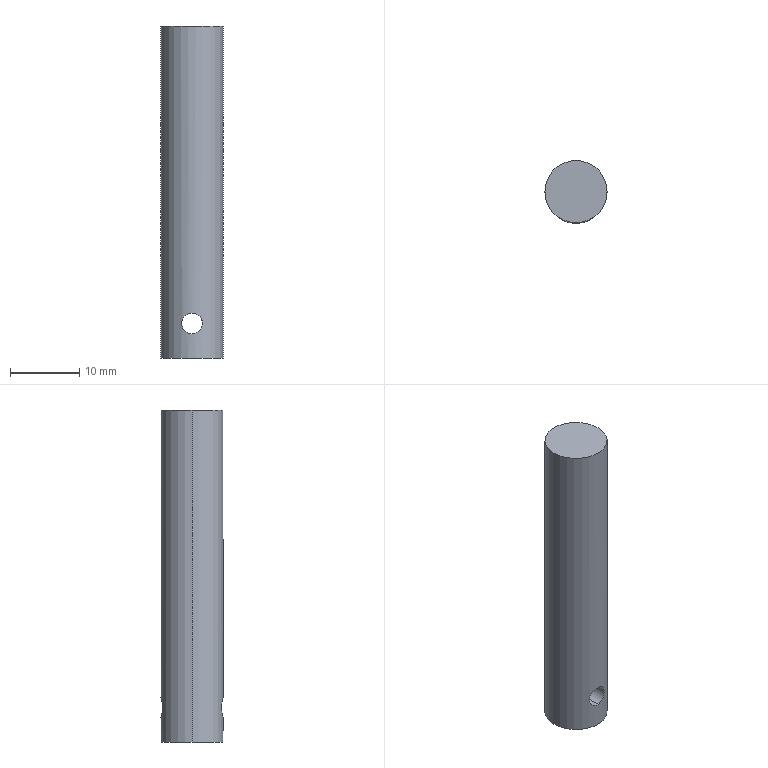Part | STEP file | Locking lead screw SGN-2-30 | 1 solid | 6 faces | box 9 x 9 x 48 mm | volume 2991 mm3 | cylinder 4 | plane 2 | commonest cylinder face diameters 3 x2 9 x2
STEP:
#1=CARTESIAN_POINT('',(0.,0.,0.));
#2=DIRECTION('',(0.,0.,1.));
#3=DIRECTION('',(1.,0.,0.));
#4=AXIS2_PLACEMENT_3D('',#1,#2,#3);
#5=CARTESIAN_POINT('',(0.,-4.5,6.5));
#6=VERTEX_POINT('',#5);
#7=CARTESIAN_POINT('',(0.,4.5,6.5));
#8=VERTEX_POINT('',#7);
#9=CARTESIAN_POINT('',(0.,-15.,6.5));
#10=DIRECTION('',(0.,1.,0.));
#11=VECTOR('',#10,1.);
#12=LINE('',#9,#11);
#13=CARTESIAN_POINT('',(0.,-15.,5.));
#14=DIRECTION('',(0.,1.,0.));
#15=DIRECTION('',(0.,0.,1.));
#16=AXIS2_PLACEMENT_3D('',#13,#14,#15);
#17=CYLINDRICAL_SURFACE('',#16,1.5);
#18=CARTESIAN_POINT('',(6.283,0.));
#19=DIRECTION('',(0.,1.));
#20=VECTOR('',#19,1.);
#21=LINE('',#18,#20);
#22=(GEOMETRIC_REPRESENTATION_CONTEXT(2)PARAMETRIC_REPRESENTATION_CONTEXT()REPRESENTATION_CONTEXT('',''));
#23=DEFINITIONAL_REPRESENTATION('',(#21),#22);
#24=PCURVE('',#17,#23);
#25=CARTESIAN_POINT('',(0.,-15.,5.));
#26=DIRECTION('',(0.,1.,0.));
#27=DIRECTION('',(0.,0.,1.));
#28=AXIS2_PLACEMENT_3D('',#25,#26,#27);
#29=CYLINDRICAL_SURFACE('',#28,1.5);
#30=CARTESIAN_POINT('',(0.,0.));
#31=DIRECTION('',(0.,1.));
#32=VECTOR('',#31,1.);
#33=LINE('',#30,#32);
#34=(GEOMETRIC_REPRESENTATION_CONTEXT(2)PARAMETRIC_REPRESENTATION_CONTEXT()REPRESENTATION_CONTEXT('',''));
#35=DEFINITIONAL_REPRESENTATION('',(#33),#34);
#36=PCURVE('',#29,#35);
#37=SURFACE_CURVE('',#12,(#24,#36),.PCURVE_S1.);
#38=EDGE_CURVE('',#6,#8,#37,.T.);
#39=ORIENTED_EDGE('',*,*,#38,.T.);
#40=CARTESIAN_POINT('',(0.,4.5,3.5));
#41=VERTEX_POINT('',#40);
#42=CARTESIAN_POINT('',(0.,4.5,6.5));
#43=CARTESIAN_POINT('',(-0.09988,4.5,6.5));
#44=CARTESIAN_POINT('',(-0.198,4.497,6.49));
#45=CARTESIAN_POINT('',(-0.3907,4.484,6.452));
#46=CARTESIAN_POINT('',(-0.4864,4.475,6.422));
#47=CARTESIAN_POINT('',(-0.7584,4.439,6.309));
#48=CARTESIAN_POINT('',(-0.9239,4.406,6.198));
#49=CARTESIAN_POINT('',(-1.198,4.34,5.923));
#50=CARTESIAN_POINT('',(-1.31,4.306,5.757));
#51=CARTESIAN_POINT('',(-1.46,4.257,5.396));
#52=CARTESIAN_POINT('',(-1.5,4.243,5.198));
#53=CARTESIAN_POINT('',(-1.5,4.243,4.902));
#54=CARTESIAN_POINT('',(-1.49,4.246,4.802));
#55=CARTESIAN_POINT('',(-1.451,4.26,4.609));
#56=CARTESIAN_POINT('',(-1.423,4.269,4.515));
#57=CARTESIAN_POINT('',(-1.309,4.306,4.241));
#58=CARTESIAN_POINT('',(-1.198,4.34,4.077));
#59=CARTESIAN_POINT('',(-0.9912,4.39,3.87));
#60=CARTESIAN_POINT('',(-0.9162,4.407,3.808));
#61=CARTESIAN_POINT('',(-0.7541,4.437,3.7));
#62=CARTESIAN_POINT('',(-0.6663,4.451,3.653));
#63=CARTESIAN_POINT('',(-0.3954,4.486,3.54));
#64=CARTESIAN_POINT('',(-0.1968,4.5,3.5));
#65=CARTESIAN_POINT('',(0.,4.5,3.5));
#66=B_SPLINE_CURVE_WITH_KNOTS('',3,(#42,#43,#44,#45,#46,#47,#48,#49,#50,#51,#52,#53,#54,#55,#56,#57,#58,#59,#60,#61,#62,#63,#64,#65),.UNSPECIFIED.,.F.,.F.,(4,2,2,2,2,2,2,2,2,2,2,4),(0.,0.0002952,0.0005905,0.001181,0.001771,0.002362,0.002657,0.002952,0.003543,0.003838,0.004133,0.004724),.UNSPECIFIED.);
#67=CARTESIAN_POINT('',(6.283,19.5));
#68=CARTESIAN_POINT('',(6.259,19.5));
#69=CARTESIAN_POINT('',(6.211,19.499));
#70=CARTESIAN_POINT('',(6.139,19.495));
#71=CARTESIAN_POINT('',(6.068,19.489));
#72=CARTESIAN_POINT('',(5.996,19.48));
#73=CARTESIAN_POINT('',(5.924,19.469));
#74=CARTESIAN_POINT('',(5.853,19.457));
#75=CARTESIAN_POINT('',(5.781,19.442));
#76=CARTESIAN_POINT('',(5.71,19.426));
#77=CARTESIAN_POINT('',(5.639,19.409));
#78=CARTESIAN_POINT('',(5.568,19.391));
#79=CARTESIAN_POINT('',(5.497,19.373));
#80=CARTESIAN_POINT('',(5.427,19.355));
#81=CARTESIAN_POINT('',(5.356,19.337));
#82=CARTESIAN_POINT('',(5.285,19.32));
#83=CARTESIAN_POINT('',(5.213,19.303));
#84=CARTESIAN_POINT('',(5.142,19.288));
#85=CARTESIAN_POINT('',(5.071,19.275));
#86=CARTESIAN_POINT('',(5.,19.264));
#87=CARTESIAN_POINT('',(4.928,19.255));
#88=CARTESIAN_POINT('',(4.857,19.248));
#89=CARTESIAN_POINT('',(4.785,19.244));
#90=CARTESIAN_POINT('',(4.713,19.242));
#91=CARTESIAN_POINT('',(4.641,19.244));
#92=CARTESIAN_POINT('',(4.568,19.248));
#93=CARTESIAN_POINT('',(4.497,19.254));
#94=CARTESIAN_POINT('',(4.425,19.263));
#95=CARTESIAN_POINT('',(4.354,19.275));
#96=CARTESIAN_POINT('',(4.282,19.288));
#97=CARTESIAN_POINT('',(4.211,19.303));
#98=CARTESIAN_POINT('',(4.139,19.32));
#99=CARTESIAN_POINT('',(4.068,19.337));
#100=CARTESIAN_POINT('',(3.998,19.355));
#101=CARTESIAN_POINT('',(3.927,19.373));
#102=CARTESIAN_POINT('',(3.856,19.392));
#103=CARTESIAN_POINT('',(3.785,19.409));
#104=CARTESIAN_POINT('',(3.714,19.426));
#105=CARTESIAN_POINT('',(3.643,19.442));
#106=CARTESIAN_POINT('',(3.571,19.457));
#107=CARTESIAN_POINT('',(3.5,19.469));
#108=CARTESIAN_POINT('',(3.429,19.48));
#109=CARTESIAN_POINT('',(3.357,19.489));
#110=CARTESIAN_POINT('',(3.285,19.495));
#111=CARTESIAN_POINT('',(3.213,19.499));
#112=CARTESIAN_POINT('',(3.165,19.5));
#113=CARTESIAN_POINT('',(3.142,19.5));
#114=B_SPLINE_CURVE_WITH_KNOTS('',3,(#67,#68,#69,#70,#71,#72,#73,#74,#75,#76,#77,#78,#79,#80,#81,#82,#83,#84,#85,#86,#87,#88,#89,#90,#91,#92,#93,#94,#95,#96,#97,#98,#99,#100,#101,#102,#103,#104,#105,#106,#107,#108,#109,#110,#111,#112,#113),.UNSPECIFIED.,.F.,.F.,(4,1,1,1,1,1,1,1,1,1,1,1,1,1,1,1,1,1,1,1,1,1,1,1,1,1,1,1,1,1,1,1,1,1,1,1,1,1,1,1,1,1,1,1,4),(0.,0.0001074,0.0002147,0.0003221,0.0004294,0.0005368,0.0006441,0.0007515,0.0008589,0.0009662,0.001074,0.001181,0.001288,0.001396,0.001503,0.00161,0.001718,0.001825,0.001932,0.00204,0.002147,0.002255,0.002362,0.002469,0.002577,0.002684,0.002791,0.002899,0.003006,0.003113,0.003221,0.003328,0.003435,0.003543,0.00365,0.003758,0.003865,0.003972,0.00408,0.004187,0.004294,0.004402,0.004509,0.004616,0.004724),.QUASI_UNIFORM_KNOTS.);
#115=(GEOMETRIC_REPRESENTATION_CONTEXT(2)PARAMETRIC_REPRESENTATION_CONTEXT()REPRESENTATION_CONTEXT('',''));
#116=DEFINITIONAL_REPRESENTATION('',(#114),#115);
#117=PCURVE('',#17,#116);
#118=CARTESIAN_POINT('',(0.,0.,48.));
#119=DIRECTION('',(0.,0.,-1.));
#120=DIRECTION('',(-1.,0.,0.));
#121=AXIS2_PLACEMENT_3D('',#118,#119,#120);
#122=CYLINDRICAL_SURFACE('',#121,4.5);
#123=CARTESIAN_POINT('',(1.571,41.5));
#124=CARTESIAN_POINT('',(1.563,41.5));
#125=CARTESIAN_POINT('',(1.547,41.503));
#126=CARTESIAN_POINT('',(1.523,41.514));
#127=CARTESIAN_POINT('',(1.499,41.533));
#128=CARTESIAN_POINT('',(1.476,41.56));
#129=CARTESIAN_POINT('',(1.453,41.595));
#130=CARTESIAN_POINT('',(1.431,41.636));
#131=CARTESIAN_POINT('',(1.41,41.684));
#132=CARTESIAN_POINT('',(1.389,41.739));
#133=CARTESIAN_POINT('',(1.369,41.8));
#134=CARTESIAN_POINT('',(1.35,41.867));
#135=CARTESIAN_POINT('',(1.333,41.939));
#136=CARTESIAN_POINT('',(1.316,42.017));
#137=CARTESIAN_POINT('',(1.301,42.1));
#138=CARTESIAN_POINT('',(1.287,42.187));
#139=CARTESIAN_POINT('',(1.274,42.279));
#140=CARTESIAN_POINT('',(1.263,42.374));
#141=CARTESIAN_POINT('',(1.253,42.472));
#142=CARTESIAN_POINT('',(1.245,42.574));
#143=CARTESIAN_POINT('',(1.239,42.678));
#144=CARTESIAN_POINT('',(1.234,42.784));
#145=CARTESIAN_POINT('',(1.232,42.892));
#146=CARTESIAN_POINT('',(1.231,42.999));
#147=CARTESIAN_POINT('',(1.232,43.107));
#148=CARTESIAN_POINT('',(1.234,43.215));
#149=CARTESIAN_POINT('',(1.239,43.321));
#150=CARTESIAN_POINT('',(1.245,43.425));
#151=CARTESIAN_POINT('',(1.253,43.527));
#152=CARTESIAN_POINT('',(1.263,43.626));
#153=CARTESIAN_POINT('',(1.274,43.722));
#154=CARTESIAN_POINT('',(1.287,43.814));
#155=CARTESIAN_POINT('',(1.301,43.901));
#156=CARTESIAN_POINT('',(1.316,43.984));
#157=CARTESIAN_POINT('',(1.333,44.062));
#158=CARTESIAN_POINT('',(1.351,44.134));
#159=CARTESIAN_POINT('',(1.369,44.201));
#160=CARTESIAN_POINT('',(1.389,44.262));
#161=CARTESIAN_POINT('',(1.41,44.316));
#162=CARTESIAN_POINT('',(1.431,44.365));
#163=CARTESIAN_POINT('',(1.453,44.406));
#164=CARTESIAN_POINT('',(1.476,44.44));
#165=CARTESIAN_POINT('',(1.499,44.466));
#166=CARTESIAN_POINT('',(1.523,44.486));
#167=CARTESIAN_POINT('',(1.547,44.497));
#168=CARTESIAN_POINT('',(1.563,44.5));
#169=CARTESIAN_POINT('',(1.571,44.5));
#170=B_SPLINE_CURVE_WITH_KNOTS('',3,(#123,#124,#125,#126,#127,#128,#129,#130,#131,#132,#133,#134,#135,#136,#137,#138,#139,#140,#141,#142,#143,#144,#145,#146,#147,#148,#149,#150,#151,#152,#153,#154,#155,#156,#157,#158,#159,#160,#161,#162,#163,#164,#165,#166,#167,#168,#169),.UNSPECIFIED.,.F.,.F.,(4,1,1,1,1,1,1,1,1,1,1,1,1,1,1,1,1,1,1,1,1,1,1,1,1,1,1,1,1,1,1,1,1,1,1,1,1,1,1,1,1,1,1,1,4),(0.,0.0001074,0.0002147,0.0003221,0.0004294,0.0005368,0.0006441,0.0007515,0.0008589,0.0009662,0.001074,0.001181,0.001288,0.001396,0.001503,0.00161,0.001718,0.001825,0.001932,0.00204,0.002147,0.002255,0.002362,0.002469,0.002577,0.002684,0.002791,0.002899,0.003006,0.003113,0.003221,0.003328,0.003435,0.003543,0.00365,0.003758,0.003865,0.003972,0.00408,0.004187,0.004294,0.004402,0.004509,0.004616,0.004724),.QUASI_UNIFORM_KNOTS.);
#171=(GEOMETRIC_REPRESENTATION_CONTEXT(2)PARAMETRIC_REPRESENTATION_CONTEXT()REPRESENTATION_CONTEXT('',''));
#172=DEFINITIONAL_REPRESENTATION('',(#170),#171);
#173=PCURVE('',#122,#172);
#174=SURFACE_CURVE('',#66,(#117,#173),.PCURVE_S1.);
#175=EDGE_CURVE('',#8,#41,#174,.T.);
#176=ORIENTED_EDGE('',*,*,#175,.T.);
#177=CARTESIAN_POINT('',(0.,-4.5,3.5));
#178=VERTEX_POINT('',#177);
#179=CARTESIAN_POINT('',(0.,-15.,3.5));
#180=DIRECTION('',(0.,1.,0.));
#181=VECTOR('',#180,1.);
#182=LINE('',#179,#181);
#183=CARTESIAN_POINT('',(3.142,0.));
#184=DIRECTION('',(0.,1.));
#185=VECTOR('',#184,1.);
#186=LINE('',#183,#185);
#187=(GEOMETRIC_REPRESENTATION_CONTEXT(2)PARAMETRIC_REPRESENTATION_CONTEXT()REPRESENTATION_CONTEXT('',''));
#188=DEFINITIONAL_REPRESENTATION('',(#186),#187);
#189=PCURVE('',#17,#188);
#190=CARTESIAN_POINT('',(3.142,0.));
#191=DIRECTION('',(0.,1.));
#192=VECTOR('',#191,1.);
#193=LINE('',#190,#192);
#194=(GEOMETRIC_REPRESENTATION_CONTEXT(2)PARAMETRIC_REPRESENTATION_CONTEXT()REPRESENTATION_CONTEXT('',''));
#195=DEFINITIONAL_REPRESENTATION('',(#193),#194);
#196=PCURVE('',#29,#195);
#197=SURFACE_CURVE('',#182,(#189,#196),.PCURVE_S1.);
#198=EDGE_CURVE('',#178,#41,#197,.T.);
#199=ORIENTED_EDGE('',*,*,#198,.F.);
#200=CARTESIAN_POINT('',(0.,-4.5,3.5));
#201=CARTESIAN_POINT('',(-0.1967,-4.5,3.5));
#202=CARTESIAN_POINT('',(-0.3953,-4.486,3.54));
#203=CARTESIAN_POINT('',(-0.6668,-4.451,3.653));
#204=CARTESIAN_POINT('',(-0.7546,-4.437,3.7));
#205=CARTESIAN_POINT('',(-0.9165,-4.406,3.809));
#206=CARTESIAN_POINT('',(-0.9916,-4.39,3.87));
#207=CARTESIAN_POINT('',(-1.199,-4.34,4.078));
#208=CARTESIAN_POINT('',(-1.309,-4.306,4.242));
#209=CARTESIAN_POINT('',(-1.423,-4.269,4.515));
#210=CARTESIAN_POINT('',(-1.451,-4.26,4.609));
#211=CARTESIAN_POINT('',(-1.49,-4.246,4.801));
#212=CARTESIAN_POINT('',(-1.5,-4.243,4.901));
#213=CARTESIAN_POINT('',(-1.5,-4.243,5.099));
#214=CARTESIAN_POINT('',(-1.49,-4.246,5.197));
#215=CARTESIAN_POINT('',(-1.452,-4.259,5.391));
#216=CARTESIAN_POINT('',(-1.422,-4.269,5.486));
#217=CARTESIAN_POINT('',(-1.31,-4.306,5.757));
#218=CARTESIAN_POINT('',(-1.198,-4.34,5.923));
#219=CARTESIAN_POINT('',(-0.9921,-4.39,6.129));
#220=CARTESIAN_POINT('',(-0.9155,-4.407,6.192));
#221=CARTESIAN_POINT('',(-0.7534,-4.437,6.301));
#222=CARTESIAN_POINT('',(-0.6676,-4.451,6.347));
#223=CARTESIAN_POINT('',(-0.4863,-4.475,6.422));
#224=CARTESIAN_POINT('',(-0.3906,-4.484,6.452));
#225=CARTESIAN_POINT('',(-0.198,-4.497,6.49));
#226=CARTESIAN_POINT('',(-0.09985,-4.5,6.5));
#227=CARTESIAN_POINT('',(0.,-4.5,6.5));
#228=B_SPLINE_CURVE_WITH_KNOTS('',3,(#200,#201,#202,#203,#204,#205,#206,#207,#208,#209,#210,#211,#212,#213,#214,#215,#216,#217,#218,#219,#220,#221,#222,#223,#224,#225,#226,#227),.UNSPECIFIED.,.F.,.F.,(4,2,2,2,2,2,2,2,2,2,2,2,2,4),(0.004724,0.005314,0.005609,0.005904,0.006495,0.00679,0.007085,0.00738,0.007675,0.008266,0.008561,0.008856,0.009151,0.009446),.UNSPECIFIED.);
#229=CARTESIAN_POINT('',(3.142,10.5));
#230=CARTESIAN_POINT('',(3.157,10.5));
#231=CARTESIAN_POINT('',(3.189,10.5));
#232=CARTESIAN_POINT('',(3.237,10.502));
#233=CARTESIAN_POINT('',(3.285,10.505));
#234=CARTESIAN_POINT('',(3.333,10.509));
#235=CARTESIAN_POINT('',(3.381,10.514));
#236=CARTESIAN_POINT('',(3.429,10.52));
#237=CARTESIAN_POINT('',(3.476,10.527));
#238=CARTESIAN_POINT('',(3.524,10.535));
#239=CARTESIAN_POINT('',(3.572,10.544));
#240=CARTESIAN_POINT('',(3.619,10.553));
#241=CARTESIAN_POINT('',(3.667,10.563));
#242=CARTESIAN_POINT('',(3.715,10.574));
#243=CARTESIAN_POINT('',(3.762,10.585));
#244=CARTESIAN_POINT('',(3.809,10.597));
#245=CARTESIAN_POINT('',(3.856,10.609));
#246=CARTESIAN_POINT('',(3.903,10.621));
#247=CARTESIAN_POINT('',(3.951,10.633));
#248=CARTESIAN_POINT('',(3.998,10.645));
#249=CARTESIAN_POINT('',(4.046,10.657));
#250=CARTESIAN_POINT('',(4.093,10.669));
#251=CARTESIAN_POINT('',(4.14,10.68));
#252=CARTESIAN_POINT('',(4.187,10.691));
#253=CARTESIAN_POINT('',(4.235,10.702));
#254=CARTESIAN_POINT('',(4.282,10.712));
#255=CARTESIAN_POINT('',(4.33,10.721));
#256=CARTESIAN_POINT('',(4.378,10.729));
#257=CARTESIAN_POINT('',(4.425,10.736));
#258=CARTESIAN_POINT('',(4.473,10.743));
#259=CARTESIAN_POINT('',(4.52,10.748));
#260=CARTESIAN_POINT('',(4.568,10.752));
#261=CARTESIAN_POINT('',(4.616,10.755));
#262=CARTESIAN_POINT('',(4.664,10.757));
#263=CARTESIAN_POINT('',(4.713,10.758));
#264=CARTESIAN_POINT('',(4.76,10.757));
#265=CARTESIAN_POINT('',(4.808,10.755));
#266=CARTESIAN_POINT('',(4.856,10.752));
#267=CARTESIAN_POINT('',(4.904,10.748));
#268=CARTESIAN_POINT('',(4.951,10.743));
#269=CARTESIAN_POINT('',(4.999,10.736));
#270=CARTESIAN_POINT('',(5.047,10.729));
#271=CARTESIAN_POINT('',(5.095,10.721));
#272=CARTESIAN_POINT('',(5.142,10.712));
#273=CARTESIAN_POINT('',(5.19,10.702));
#274=CARTESIAN_POINT('',(5.237,10.691));
#275=CARTESIAN_POINT('',(5.285,10.68));
#276=CARTESIAN_POINT('',(5.332,10.669));
#277=CARTESIAN_POINT('',(5.38,10.657));
#278=CARTESIAN_POINT('',(5.427,10.645));
#279=CARTESIAN_POINT('',(5.474,10.633));
#280=CARTESIAN_POINT('',(5.521,10.621));
#281=CARTESIAN_POINT('',(5.569,10.609));
#282=CARTESIAN_POINT('',(5.616,10.597));
#283=CARTESIAN_POINT('',(5.664,10.585));
#284=CARTESIAN_POINT('',(5.711,10.574));
#285=CARTESIAN_POINT('',(5.758,10.563));
#286=CARTESIAN_POINT('',(5.805,10.553));
#287=CARTESIAN_POINT('',(5.853,10.544));
#288=CARTESIAN_POINT('',(5.9,10.535));
#289=CARTESIAN_POINT('',(5.948,10.527));
#290=CARTESIAN_POINT('',(5.996,10.52));
#291=CARTESIAN_POINT('',(6.044,10.514));
#292=CARTESIAN_POINT('',(6.092,10.509));
#293=CARTESIAN_POINT('',(6.139,10.505));
#294=CARTESIAN_POINT('',(6.187,10.502));
#295=CARTESIAN_POINT('',(6.235,10.5));
#296=CARTESIAN_POINT('',(6.267,10.5));
#297=CARTESIAN_POINT('',(6.283,10.5));
#298=B_SPLINE_CURVE_WITH_KNOTS('',3,(#229,#230,#231,#232,#233,#234,#235,#236,#237,#238,#239,#240,#241,#242,#243,#244,#245,#246,#247,#248,#249,#250,#251,#252,#253,#254,#255,#256,#257,#258,#259,#260,#261,#262,#263,#264,#265,#266,#267,#268,#269,#270,#271,#272,#273,#274,#275,#276,#277,#278,#279,#280,#281,#282,#283,#284,#285,#286,#287,#288,#289,#290,#291,#292,#293,#294,#295,#296,#297),.UNSPECIFIED.,.F.,.F.,(4,1,1,1,1,1,1,1,1,1,1,1,1,1,1,1,1,1,1,1,1,1,1,1,1,1,1,1,1,1,1,1,1,1,1,1,1,1,1,1,1,1,1,1,1,1,1,1,1,1,1,1,1,1,1,1,1,1,1,1,1,1,1,1,1,1,4),(0.004724,0.004795,0.004867,0.004938,0.00501,0.005082,0.005153,0.005225,0.005296,0.005368,0.005439,0.005511,0.005582,0.005654,0.005725,0.005797,0.005869,0.00594,0.006012,0.006083,0.006155,0.006226,0.006298,0.006369,0.006441,0.006513,0.006584,0.006656,0.006727,0.006799,0.00687,0.006942,0.007013,0.007085,0.007157,0.007228,0.0073,0.007371,0.007443,0.007514,0.007586,0.007657,0.007729,0.007801,0.007872,0.007944,0.008015,0.008087,0.008158,0.00823,0.008301,0.008373,0.008445,0.008516,0.008588,0.008659,0.008731,0.008802,0.008874,0.008945,0.009017,0.009089,0.00916,0.009232,0.009303,0.009375,0.009446),.QUASI_UNIFORM_KNOTS.);
#299=(GEOMETRIC_REPRESENTATION_CONTEXT(2)PARAMETRIC_REPRESENTATION_CONTEXT()REPRESENTATION_CONTEXT('',''));
#300=DEFINITIONAL_REPRESENTATION('',(#298),#299);
#301=PCURVE('',#17,#300);
#302=CARTESIAN_POINT('',(0.,0.,48.));
#303=DIRECTION('',(0.,0.,-1.));
#304=DIRECTION('',(-1.,0.,0.));
#305=AXIS2_PLACEMENT_3D('',#302,#303,#304);
#306=CYLINDRICAL_SURFACE('',#305,4.5);
#307=CARTESIAN_POINT('',(4.712,44.5));
#308=CARTESIAN_POINT('',(4.718,44.5));
#309=CARTESIAN_POINT('',(4.728,44.499));
#310=CARTESIAN_POINT('',(4.744,44.494));
#311=CARTESIAN_POINT('',(4.76,44.485));
#312=CARTESIAN_POINT('',(4.776,44.473));
#313=CARTESIAN_POINT('',(4.791,44.458));
#314=CARTESIAN_POINT('',(4.807,44.439));
#315=CARTESIAN_POINT('',(4.822,44.417));
#316=CARTESIAN_POINT('',(4.837,44.392));
#317=CARTESIAN_POINT('',(4.852,44.364));
#318=CARTESIAN_POINT('',(4.866,44.332));
#319=CARTESIAN_POINT('',(4.88,44.298));
#320=CARTESIAN_POINT('',(4.894,44.261));
#321=CARTESIAN_POINT('',(4.907,44.221));
#322=CARTESIAN_POINT('',(4.92,44.179));
#323=CARTESIAN_POINT('',(4.933,44.133));
#324=CARTESIAN_POINT('',(4.945,44.086));
#325=CARTESIAN_POINT('',(4.956,44.035));
#326=CARTESIAN_POINT('',(4.967,43.983));
#327=CARTESIAN_POINT('',(4.978,43.928));
#328=CARTESIAN_POINT('',(4.987,43.871));
#329=CARTESIAN_POINT('',(4.997,43.813));
#330=CARTESIAN_POINT('',(5.005,43.752));
#331=CARTESIAN_POINT('',(5.013,43.69));
#332=CARTESIAN_POINT('',(5.02,43.626));
#333=CARTESIAN_POINT('',(5.027,43.56));
#334=CARTESIAN_POINT('',(5.033,43.493));
#335=CARTESIAN_POINT('',(5.038,43.425));
#336=CARTESIAN_POINT('',(5.042,43.356));
#337=CARTESIAN_POINT('',(5.046,43.286));
#338=CARTESIAN_POINT('',(5.049,43.216));
#339=CARTESIAN_POINT('',(5.051,43.144));
#340=CARTESIAN_POINT('',(5.052,43.072));
#341=CARTESIAN_POINT('',(5.052,43.));
#342=CARTESIAN_POINT('',(5.052,42.928));
#343=CARTESIAN_POINT('',(5.051,42.857));
#344=CARTESIAN_POINT('',(5.049,42.786));
#345=CARTESIAN_POINT('',(5.046,42.715));
#346=CARTESIAN_POINT('',(5.042,42.645));
#347=CARTESIAN_POINT('',(5.038,42.575));
#348=CARTESIAN_POINT('',(5.033,42.507));
#349=CARTESIAN_POINT('',(5.027,42.44));
#350=CARTESIAN_POINT('',(5.02,42.374));
#351=CARTESIAN_POINT('',(5.013,42.31));
#352=CARTESIAN_POINT('',(5.005,42.248));
#353=CARTESIAN_POINT('',(4.996,42.187));
#354=CARTESIAN_POINT('',(4.987,42.128));
#355=CARTESIAN_POINT('',(4.977,42.072));
#356=CARTESIAN_POINT('',(4.967,42.017));
#357=CARTESIAN_POINT('',(4.956,41.964));
#358=CARTESIAN_POINT('',(4.945,41.914));
#359=CARTESIAN_POINT('',(4.933,41.867));
#360=CARTESIAN_POINT('',(4.92,41.821));
#361=CARTESIAN_POINT('',(4.907,41.778));
#362=CARTESIAN_POINT('',(4.894,41.738));
#363=CARTESIAN_POINT('',(4.88,41.702));
#364=CARTESIAN_POINT('',(4.866,41.667));
#365=CARTESIAN_POINT('',(4.852,41.636));
#366=CARTESIAN_POINT('',(4.837,41.608));
#367=CARTESIAN_POINT('',(4.822,41.583));
#368=CARTESIAN_POINT('',(4.807,41.561));
#369=CARTESIAN_POINT('',(4.791,41.542));
#370=CARTESIAN_POINT('',(4.776,41.527));
#371=CARTESIAN_POINT('',(4.76,41.515));
#372=CARTESIAN_POINT('',(4.744,41.506));
#373=CARTESIAN_POINT('',(4.728,41.501));
#374=CARTESIAN_POINT('',(4.718,41.5));
#375=CARTESIAN_POINT('',(4.712,41.5));
#376=B_SPLINE_CURVE_WITH_KNOTS('',3,(#307,#308,#309,#310,#311,#312,#313,#314,#315,#316,#317,#318,#319,#320,#321,#322,#323,#324,#325,#326,#327,#328,#329,#330,#331,#332,#333,#334,#335,#336,#337,#338,#339,#340,#341,#342,#343,#344,#345,#346,#347,#348,#349,#350,#351,#352,#353,#354,#355,#356,#357,#358,#359,#360,#361,#362,#363,#364,#365,#366,#367,#368,#369,#370,#371,#372,#373,#374,#375),.UNSPECIFIED.,.F.,.F.,(4,1,1,1,1,1,1,1,1,1,1,1,1,1,1,1,1,1,1,1,1,1,1,1,1,1,1,1,1,1,1,1,1,1,1,1,1,1,1,1,1,1,1,1,1,1,1,1,1,1,1,1,1,1,1,1,1,1,1,1,1,1,1,1,1,1,4),(0.004724,0.004795,0.004867,0.004938,0.00501,0.005082,0.005153,0.005225,0.005296,0.005368,0.005439,0.005511,0.005582,0.005654,0.005725,0.005797,0.005869,0.00594,0.006012,0.006083,0.006155,0.006226,0.006298,0.006369,0.006441,0.006513,0.006584,0.006656,0.006727,0.006799,0.00687,0.006942,0.007013,0.007085,0.007157,0.007228,0.0073,0.007371,0.007443,0.007514,0.007586,0.007657,0.007729,0.007801,0.007872,0.007944,0.008015,0.008087,0.008158,0.00823,0.008301,0.008373,0.008445,0.008516,0.008588,0.008659,0.008731,0.008802,0.008874,0.008945,0.009017,0.009089,0.00916,0.009232,0.009303,0.009375,0.009446),.QUASI_UNIFORM_KNOTS.);
#377=(GEOMETRIC_REPRESENTATION_CONTEXT(2)PARAMETRIC_REPRESENTATION_CONTEXT()REPRESENTATION_CONTEXT('',''));
#378=DEFINITIONAL_REPRESENTATION('',(#376),#377);
#379=PCURVE('',#306,#378);
#380=SURFACE_CURVE('',#228,(#301,#379),.PCURVE_S1.);
#381=EDGE_CURVE('',#178,#6,#380,.T.);
#382=ORIENTED_EDGE('',*,*,#381,.T.);
#383=EDGE_LOOP('',(#39,#176,#199,#382));
#384=FACE_BOUND('',#383,.F.);
#385=ADVANCED_FACE('',(#384),#17,.F.);
#386=ORIENTED_EDGE('',*,*,#175,.T.);
#387=CARTESIAN_POINT('',(0.,4.5,3.5));
#388=CARTESIAN_POINT('',(0.1967,4.5,3.5));
#389=CARTESIAN_POINT('',(0.3953,4.486,3.54));
#390=CARTESIAN_POINT('',(0.6668,4.451,3.653));
#391=CARTESIAN_POINT('',(0.7546,4.437,3.7));
#392=CARTESIAN_POINT('',(0.9165,4.406,3.809));
#393=CARTESIAN_POINT('',(0.9916,4.39,3.87));
#394=CARTESIAN_POINT('',(1.199,4.34,4.078));
#395=CARTESIAN_POINT('',(1.309,4.306,4.242));
#396=CARTESIAN_POINT('',(1.423,4.269,4.515));
#397=CARTESIAN_POINT('',(1.451,4.26,4.609));
#398=CARTESIAN_POINT('',(1.49,4.246,4.801));
#399=CARTESIAN_POINT('',(1.5,4.243,4.901));
#400=CARTESIAN_POINT('',(1.5,4.243,5.099));
#401=CARTESIAN_POINT('',(1.49,4.246,5.197));
#402=CARTESIAN_POINT('',(1.452,4.259,5.391));
#403=CARTESIAN_POINT('',(1.422,4.269,5.486));
#404=CARTESIAN_POINT('',(1.31,4.306,5.757));
#405=CARTESIAN_POINT('',(1.198,4.34,5.923));
#406=CARTESIAN_POINT('',(0.9921,4.39,6.129));
#407=CARTESIAN_POINT('',(0.9155,4.407,6.192));
#408=CARTESIAN_POINT('',(0.7534,4.437,6.301));
#409=CARTESIAN_POINT('',(0.6676,4.451,6.347));
#410=CARTESIAN_POINT('',(0.4863,4.475,6.422));
#411=CARTESIAN_POINT('',(0.3906,4.484,6.452));
#412=CARTESIAN_POINT('',(0.198,4.497,6.49));
#413=CARTESIAN_POINT('',(0.09985,4.5,6.5));
#414=CARTESIAN_POINT('',(0.,4.5,6.5));
#415=B_SPLINE_CURVE_WITH_KNOTS('',3,(#387,#388,#389,#390,#391,#392,#393,#394,#395,#396,#397,#398,#399,#400,#401,#402,#403,#404,#405,#406,#407,#408,#409,#410,#411,#412,#413,#414),.UNSPECIFIED.,.F.,.F.,(4,2,2,2,2,2,2,2,2,2,2,2,2,4),(0.004724,0.005314,0.005609,0.005904,0.006495,0.00679,0.007085,0.00738,0.007675,0.008266,0.008561,0.008856,0.009151,0.009446),.UNSPECIFIED.);
#416=CARTESIAN_POINT('',(1.571,44.5));
#417=CARTESIAN_POINT('',(1.576,44.5));
#418=CARTESIAN_POINT('',(1.587,44.499));
#419=CARTESIAN_POINT('',(1.603,44.494));
#420=CARTESIAN_POINT('',(1.618,44.485));
#421=CARTESIAN_POINT('',(1.634,44.473));
#422=CARTESIAN_POINT('',(1.65,44.458));
#423=CARTESIAN_POINT('',(1.665,44.439));
#424=CARTESIAN_POINT('',(1.681,44.417));
#425=CARTESIAN_POINT('',(1.696,44.392));
#426=CARTESIAN_POINT('',(1.71,44.364));
#427=CARTESIAN_POINT('',(1.725,44.332));
#428=CARTESIAN_POINT('',(1.739,44.298));
#429=CARTESIAN_POINT('',(1.753,44.261));
#430=CARTESIAN_POINT('',(1.766,44.221));
#431=CARTESIAN_POINT('',(1.779,44.179));
#432=CARTESIAN_POINT('',(1.791,44.133));
#433=CARTESIAN_POINT('',(1.803,44.086));
#434=CARTESIAN_POINT('',(1.815,44.035));
#435=CARTESIAN_POINT('',(1.826,43.983));
#436=CARTESIAN_POINT('',(1.836,43.928));
#437=CARTESIAN_POINT('',(1.846,43.871));
#438=CARTESIAN_POINT('',(1.855,43.813));
#439=CARTESIAN_POINT('',(1.864,43.752));
#440=CARTESIAN_POINT('',(1.871,43.69));
#441=CARTESIAN_POINT('',(1.879,43.626));
#442=CARTESIAN_POINT('',(1.885,43.56));
#443=CARTESIAN_POINT('',(1.891,43.493));
#444=CARTESIAN_POINT('',(1.896,43.425));
#445=CARTESIAN_POINT('',(1.901,43.356));
#446=CARTESIAN_POINT('',(1.904,43.286));
#447=CARTESIAN_POINT('',(1.907,43.216));
#448=CARTESIAN_POINT('',(1.909,43.144));
#449=CARTESIAN_POINT('',(1.91,43.072));
#450=CARTESIAN_POINT('',(1.911,43.));
#451=CARTESIAN_POINT('',(1.91,42.928));
#452=CARTESIAN_POINT('',(1.909,42.857));
#453=CARTESIAN_POINT('',(1.907,42.786));
#454=CARTESIAN_POINT('',(1.904,42.715));
#455=CARTESIAN_POINT('',(1.901,42.645));
#456=CARTESIAN_POINT('',(1.896,42.575));
#457=CARTESIAN_POINT('',(1.891,42.507));
#458=CARTESIAN_POINT('',(1.885,42.44));
#459=CARTESIAN_POINT('',(1.879,42.374));
#460=CARTESIAN_POINT('',(1.871,42.31));
#461=CARTESIAN_POINT('',(1.863,42.248));
#462=CARTESIAN_POINT('',(1.855,42.187));
#463=CARTESIAN_POINT('',(1.846,42.128));
#464=CARTESIAN_POINT('',(1.836,42.072));
#465=CARTESIAN_POINT('',(1.825,42.017));
#466=CARTESIAN_POINT('',(1.815,41.964));
#467=CARTESIAN_POINT('',(1.803,41.914));
#468=CARTESIAN_POINT('',(1.791,41.867));
#469=CARTESIAN_POINT('',(1.779,41.821));
#470=CARTESIAN_POINT('',(1.766,41.778));
#471=CARTESIAN_POINT('',(1.752,41.738));
#472=CARTESIAN_POINT('',(1.739,41.702));
#473=CARTESIAN_POINT('',(1.725,41.667));
#474=CARTESIAN_POINT('',(1.71,41.636));
#475=CARTESIAN_POINT('',(1.696,41.608));
#476=CARTESIAN_POINT('',(1.681,41.583));
#477=CARTESIAN_POINT('',(1.665,41.561));
#478=CARTESIAN_POINT('',(1.65,41.542));
#479=CARTESIAN_POINT('',(1.634,41.527));
#480=CARTESIAN_POINT('',(1.619,41.515));
#481=CARTESIAN_POINT('',(1.603,41.506));
#482=CARTESIAN_POINT('',(1.587,41.501));
#483=CARTESIAN_POINT('',(1.576,41.5));
#484=CARTESIAN_POINT('',(1.571,41.5));
#485=B_SPLINE_CURVE_WITH_KNOTS('',3,(#416,#417,#418,#419,#420,#421,#422,#423,#424,#425,#426,#427,#428,#429,#430,#431,#432,#433,#434,#435,#436,#437,#438,#439,#440,#441,#442,#443,#444,#445,#446,#447,#448,#449,#450,#451,#452,#453,#454,#455,#456,#457,#458,#459,#460,#461,#462,#463,#464,#465,#466,#467,#468,#469,#470,#471,#472,#473,#474,#475,#476,#477,#478,#479,#480,#481,#482,#483,#484),.UNSPECIFIED.,.F.,.F.,(4,1,1,1,1,1,1,1,1,1,1,1,1,1,1,1,1,1,1,1,1,1,1,1,1,1,1,1,1,1,1,1,1,1,1,1,1,1,1,1,1,1,1,1,1,1,1,1,1,1,1,1,1,1,1,1,1,1,1,1,1,1,1,1,1,1,4),(0.004724,0.004795,0.004867,0.004938,0.00501,0.005082,0.005153,0.005225,0.005296,0.005368,0.005439,0.005511,0.005582,0.005654,0.005725,0.005797,0.005869,0.00594,0.006012,0.006083,0.006155,0.006226,0.006298,0.006369,0.006441,0.006513,0.006584,0.006656,0.006727,0.006799,0.00687,0.006942,0.007013,0.007085,0.007157,0.007228,0.0073,0.007371,0.007443,0.007514,0.007586,0.007657,0.007729,0.007801,0.007872,0.007944,0.008015,0.008087,0.008158,0.00823,0.008301,0.008373,0.008445,0.008516,0.008588,0.008659,0.008731,0.008802,0.008874,0.008945,0.009017,0.009089,0.00916,0.009232,0.009303,0.009375,0.009446),.QUASI_UNIFORM_KNOTS.);
#486=(GEOMETRIC_REPRESENTATION_CONTEXT(2)PARAMETRIC_REPRESENTATION_CONTEXT()REPRESENTATION_CONTEXT('',''));
#487=DEFINITIONAL_REPRESENTATION('',(#485),#486);
#488=PCURVE('',#122,#487);
#489=CARTESIAN_POINT('',(3.142,19.5));
#490=CARTESIAN_POINT('',(3.126,19.5));
#491=CARTESIAN_POINT('',(3.094,19.5));
#492=CARTESIAN_POINT('',(3.046,19.498));
#493=CARTESIAN_POINT('',(2.998,19.495));
#494=CARTESIAN_POINT('',(2.95,19.491));
#495=CARTESIAN_POINT('',(2.902,19.486));
#496=CARTESIAN_POINT('',(2.854,19.48));
#497=CARTESIAN_POINT('',(2.807,19.473));
#498=CARTESIAN_POINT('',(2.759,19.465));
#499=CARTESIAN_POINT('',(2.712,19.456));
#500=CARTESIAN_POINT('',(2.664,19.447));
#501=CARTESIAN_POINT('',(2.616,19.437));
#502=CARTESIAN_POINT('',(2.568,19.426));
#503=CARTESIAN_POINT('',(2.521,19.415));
#504=CARTESIAN_POINT('',(2.474,19.403));
#505=CARTESIAN_POINT('',(2.427,19.391));
#506=CARTESIAN_POINT('',(2.38,19.379));
#507=CARTESIAN_POINT('',(2.332,19.367));
#508=CARTESIAN_POINT('',(2.285,19.355));
#509=CARTESIAN_POINT('',(2.238,19.343));
#510=CARTESIAN_POINT('',(2.19,19.331));
#511=CARTESIAN_POINT('',(2.143,19.32));
#512=CARTESIAN_POINT('',(2.096,19.309));
#513=CARTESIAN_POINT('',(2.048,19.298));
#514=CARTESIAN_POINT('',(2.001,19.288));
#515=CARTESIAN_POINT('',(1.953,19.279));
#516=CARTESIAN_POINT('',(1.905,19.271));
#517=CARTESIAN_POINT('',(1.858,19.264));
#518=CARTESIAN_POINT('',(1.81,19.257));
#519=CARTESIAN_POINT('',(1.763,19.252));
#520=CARTESIAN_POINT('',(1.715,19.248));
#521=CARTESIAN_POINT('',(1.667,19.245));
#522=CARTESIAN_POINT('',(1.619,19.243));
#523=CARTESIAN_POINT('',(1.571,19.242));
#524=CARTESIAN_POINT('',(1.523,19.243));
#525=CARTESIAN_POINT('',(1.475,19.245));
#526=CARTESIAN_POINT('',(1.427,19.248));
#527=CARTESIAN_POINT('',(1.38,19.252));
#528=CARTESIAN_POINT('',(1.332,19.257));
#529=CARTESIAN_POINT('',(1.284,19.264));
#530=CARTESIAN_POINT('',(1.236,19.271));
#531=CARTESIAN_POINT('',(1.188,19.279));
#532=CARTESIAN_POINT('',(1.141,19.288));
#533=CARTESIAN_POINT('',(1.093,19.298));
#534=CARTESIAN_POINT('',(1.046,19.309));
#535=CARTESIAN_POINT('',(0.9984,19.32));
#536=CARTESIAN_POINT('',(0.951,19.331));
#537=CARTESIAN_POINT('',(0.9037,19.343));
#538=CARTESIAN_POINT('',(0.8564,19.355));
#539=CARTESIAN_POINT('',(0.8091,19.367));
#540=CARTESIAN_POINT('',(0.762,19.379));
#541=CARTESIAN_POINT('',(0.7146,19.391));
#542=CARTESIAN_POINT('',(0.667,19.403));
#543=CARTESIAN_POINT('',(0.6195,19.415));
#544=CARTESIAN_POINT('',(0.5722,19.426));
#545=CARTESIAN_POINT('',(0.525,19.437));
#546=CARTESIAN_POINT('',(0.4778,19.447));
#547=CARTESIAN_POINT('',(0.4305,19.456));
#548=CARTESIAN_POINT('',(0.383,19.465));
#549=CARTESIAN_POINT('',(0.3351,19.473));
#550=CARTESIAN_POINT('',(0.2872,19.48));
#551=CARTESIAN_POINT('',(0.2392,19.486));
#552=CARTESIAN_POINT('',(0.1915,19.491));
#553=CARTESIAN_POINT('',(0.1439,19.495));
#554=CARTESIAN_POINT('',(0.09618,19.498));
#555=CARTESIAN_POINT('',(0.04828,19.5));
#556=CARTESIAN_POINT('',(0.01614,19.5));
#557=CARTESIAN_POINT('',(0.,19.5));
#558=B_SPLINE_CURVE_WITH_KNOTS('',3,(#489,#490,#491,#492,#493,#494,#495,#496,#497,#498,#499,#500,#501,#502,#503,#504,#505,#506,#507,#508,#509,#510,#511,#512,#513,#514,#515,#516,#517,#518,#519,#520,#521,#522,#523,#524,#525,#526,#527,#528,#529,#530,#531,#532,#533,#534,#535,#536,#537,#538,#539,#540,#541,#542,#543,#544,#545,#546,#547,#548,#549,#550,#551,#552,#553,#554,#555,#556,#557),.UNSPECIFIED.,.F.,.F.,(4,1,1,1,1,1,1,1,1,1,1,1,1,1,1,1,1,1,1,1,1,1,1,1,1,1,1,1,1,1,1,1,1,1,1,1,1,1,1,1,1,1,1,1,1,1,1,1,1,1,1,1,1,1,1,1,1,1,1,1,1,1,1,1,1,1,4),(0.004724,0.004795,0.004867,0.004938,0.00501,0.005082,0.005153,0.005225,0.005296,0.005368,0.005439,0.005511,0.005582,0.005654,0.005725,0.005797,0.005869,0.00594,0.006012,0.006083,0.006155,0.006226,0.006298,0.006369,0.006441,0.006513,0.006584,0.006656,0.006727,0.006799,0.00687,0.006942,0.007013,0.007085,0.007157,0.007228,0.0073,0.007371,0.007443,0.007514,0.007586,0.007657,0.007729,0.007801,0.007872,0.007944,0.008015,0.008087,0.008158,0.00823,0.008301,0.008373,0.008445,0.008516,0.008588,0.008659,0.008731,0.008802,0.008874,0.008945,0.009017,0.009089,0.00916,0.009232,0.009303,0.009375,0.009446),.QUASI_UNIFORM_KNOTS.);
#559=(GEOMETRIC_REPRESENTATION_CONTEXT(2)PARAMETRIC_REPRESENTATION_CONTEXT()REPRESENTATION_CONTEXT('',''));
#560=DEFINITIONAL_REPRESENTATION('',(#558),#559);
#561=PCURVE('',#29,#560);
#562=SURFACE_CURVE('',#415,(#488,#561),.PCURVE_S1.);
#563=EDGE_CURVE('',#41,#8,#562,.T.);
#564=ORIENTED_EDGE('',*,*,#563,.T.);
#565=EDGE_LOOP('',(#386,#564));
#566=FACE_BOUND('',#565,.T.);
#567=CARTESIAN_POINT('',(4.5,0.,48.));
#568=VERTEX_POINT('',#567);
#569=CARTESIAN_POINT('',(-4.5,0.,48.));
#570=VERTEX_POINT('',#569);
#571=CARTESIAN_POINT('',(0.,0.,48.));
#572=DIRECTION('',(0.,0.,1.));
#573=DIRECTION('',(1.,0.,0.));
#574=AXIS2_PLACEMENT_3D('',#571,#572,#573);
#575=CIRCLE('',#574,4.5);
#576=CARTESIAN_POINT('',(3.142,0.));
#577=DIRECTION('',(-1.,0.));
#578=VECTOR('',#577,1.);
#579=LINE('',#576,#578);
#580=(GEOMETRIC_REPRESENTATION_CONTEXT(2)PARAMETRIC_REPRESENTATION_CONTEXT()REPRESENTATION_CONTEXT('',''));
#581=DEFINITIONAL_REPRESENTATION('',(#579),#580);
#582=PCURVE('',#122,#581);
#583=CARTESIAN_POINT('',(0.,0.,48.));
#584=DIRECTION('',(0.,0.,1.));
#585=DIRECTION('',(1.,0.,0.));
#586=AXIS2_PLACEMENT_3D('',#583,#584,#585);
#587=PLANE('',#586);
#588=CARTESIAN_POINT('',(0.,0.));
#589=DIRECTION('',(1.,0.));
#590=AXIS2_PLACEMENT_2D('',#588,#589);
#591=CIRCLE('',#590,4.5);
#592=(GEOMETRIC_REPRESENTATION_CONTEXT(2)PARAMETRIC_REPRESENTATION_CONTEXT()REPRESENTATION_CONTEXT('',''));
#593=DEFINITIONAL_REPRESENTATION('',(#591),#592);
#594=PCURVE('',#587,#593);
#595=SURFACE_CURVE('',#575,(#582,#594),.PCURVE_S1.);
#596=EDGE_CURVE('',#568,#570,#595,.T.);
#597=ORIENTED_EDGE('',*,*,#596,.F.);
#598=CARTESIAN_POINT('',(4.5,0.,0.));
#599=VERTEX_POINT('',#598);
#600=CARTESIAN_POINT('',(4.5,0.,48.));
#601=DIRECTION('',(0.,0.,-1.));
#602=VECTOR('',#601,1.);
#603=LINE('',#600,#602);
#604=CARTESIAN_POINT('',(3.142,0.));
#605=DIRECTION('',(0.,1.));
#606=VECTOR('',#605,1.);
#607=LINE('',#604,#606);
#608=(GEOMETRIC_REPRESENTATION_CONTEXT(2)PARAMETRIC_REPRESENTATION_CONTEXT()REPRESENTATION_CONTEXT('',''));
#609=DEFINITIONAL_REPRESENTATION('',(#607),#608);
#610=PCURVE('',#122,#609);
#611=CARTESIAN_POINT('',(3.142,0.));
#612=DIRECTION('',(0.,1.));
#613=VECTOR('',#612,1.);
#614=LINE('',#611,#613);
#615=(GEOMETRIC_REPRESENTATION_CONTEXT(2)PARAMETRIC_REPRESENTATION_CONTEXT()REPRESENTATION_CONTEXT('',''));
#616=DEFINITIONAL_REPRESENTATION('',(#614),#615);
#617=PCURVE('',#306,#616);
#618=SURFACE_CURVE('',#603,(#610,#617),.PCURVE_S1.);
#619=EDGE_CURVE('',#568,#599,#618,.T.);
#620=ORIENTED_EDGE('',*,*,#619,.T.);
#621=CARTESIAN_POINT('',(-4.5,0.,0.));
#622=VERTEX_POINT('',#621);
#623=CARTESIAN_POINT('',(0.,0.,0.));
#624=DIRECTION('',(0.,0.,1.));
#625=DIRECTION('',(1.,0.,0.));
#626=AXIS2_PLACEMENT_3D('',#623,#624,#625);
#627=CIRCLE('',#626,4.5);
#628=CARTESIAN_POINT('',(3.142,48.));
#629=DIRECTION('',(-1.,0.));
#630=VECTOR('',#629,1.);
#631=LINE('',#628,#630);
#632=(GEOMETRIC_REPRESENTATION_CONTEXT(2)PARAMETRIC_REPRESENTATION_CONTEXT()REPRESENTATION_CONTEXT('',''));
#633=DEFINITIONAL_REPRESENTATION('',(#631),#632);
#634=PCURVE('',#122,#633);
#635=CARTESIAN_POINT('',(0.,0.,0.));
#636=DIRECTION('',(0.,0.,1.));
#637=DIRECTION('',(1.,0.,0.));
#638=AXIS2_PLACEMENT_3D('',#635,#636,#637);
#639=PLANE('',#638);
#640=CARTESIAN_POINT('',(0.,0.));
#641=DIRECTION('',(1.,0.));
#642=AXIS2_PLACEMENT_2D('',#640,#641);
#643=CIRCLE('',#642,4.5);
#644=(GEOMETRIC_REPRESENTATION_CONTEXT(2)PARAMETRIC_REPRESENTATION_CONTEXT()REPRESENTATION_CONTEXT('',''));
#645=DEFINITIONAL_REPRESENTATION('',(#643),#644);
#646=PCURVE('',#639,#645);
#647=SURFACE_CURVE('',#627,(#634,#646),.PCURVE_S1.);
#648=EDGE_CURVE('',#599,#622,#647,.T.);
#649=ORIENTED_EDGE('',*,*,#648,.T.);
#650=CARTESIAN_POINT('',(-4.5,0.,48.));
#651=DIRECTION('',(0.,0.,-1.));
#652=VECTOR('',#651,1.);
#653=LINE('',#650,#652);
#654=CARTESIAN_POINT('',(0.,0.));
#655=DIRECTION('',(0.,1.));
#656=VECTOR('',#655,1.);
#657=LINE('',#654,#656);
#658=(GEOMETRIC_REPRESENTATION_CONTEXT(2)PARAMETRIC_REPRESENTATION_CONTEXT()REPRESENTATION_CONTEXT('',''));
#659=DEFINITIONAL_REPRESENTATION('',(#657),#658);
#660=PCURVE('',#122,#659);
#661=CARTESIAN_POINT('',(6.283,0.));
#662=DIRECTION('',(0.,1.));
#663=VECTOR('',#662,1.);
#664=LINE('',#661,#663);
#665=(GEOMETRIC_REPRESENTATION_CONTEXT(2)PARAMETRIC_REPRESENTATION_CONTEXT()REPRESENTATION_CONTEXT('',''));
#666=DEFINITIONAL_REPRESENTATION('',(#664),#665);
#667=PCURVE('',#306,#666);
#668=SURFACE_CURVE('',#653,(#660,#667),.PCURVE_S1.);
#669=EDGE_CURVE('',#570,#622,#668,.T.);
#670=ORIENTED_EDGE('',*,*,#669,.F.);
#671=EDGE_LOOP('',(#597,#620,#649,#670));
#672=FACE_BOUND('',#671,.T.);
#673=ADVANCED_FACE('',(#566,#672),#122,.T.);
#674=ORIENTED_EDGE('',*,*,#619,.F.);
#675=CARTESIAN_POINT('',(0.,0.,48.));
#676=DIRECTION('',(0.,0.,1.));
#677=DIRECTION('',(1.,0.,0.));
#678=AXIS2_PLACEMENT_3D('',#675,#676,#677);
#679=CIRCLE('',#678,4.5);
#680=CARTESIAN_POINT('',(9.425,0.));
#681=DIRECTION('',(-1.,0.));
#682=VECTOR('',#681,1.);
#683=LINE('',#680,#682);
#684=(GEOMETRIC_REPRESENTATION_CONTEXT(2)PARAMETRIC_REPRESENTATION_CONTEXT()REPRESENTATION_CONTEXT('',''));
#685=DEFINITIONAL_REPRESENTATION('',(#683),#684);
#686=PCURVE('',#306,#685);
#687=CARTESIAN_POINT('',(0.,0.));
#688=DIRECTION('',(1.,0.));
#689=AXIS2_PLACEMENT_2D('',#687,#688);
#690=CIRCLE('',#689,4.5);
#691=(GEOMETRIC_REPRESENTATION_CONTEXT(2)PARAMETRIC_REPRESENTATION_CONTEXT()REPRESENTATION_CONTEXT('',''));
#692=DEFINITIONAL_REPRESENTATION('',(#690),#691);
#693=PCURVE('',#587,#692);
#694=SURFACE_CURVE('',#679,(#686,#693),.PCURVE_S1.);
#695=EDGE_CURVE('',#570,#568,#694,.T.);
#696=ORIENTED_EDGE('',*,*,#695,.F.);
#697=ORIENTED_EDGE('',*,*,#669,.T.);
#698=CARTESIAN_POINT('',(0.,0.,0.));
#699=DIRECTION('',(0.,0.,1.));
#700=DIRECTION('',(1.,0.,0.));
#701=AXIS2_PLACEMENT_3D('',#698,#699,#700);
#702=CIRCLE('',#701,4.5);
#703=CARTESIAN_POINT('',(9.425,48.));
#704=DIRECTION('',(-1.,0.));
#705=VECTOR('',#704,1.);
#706=LINE('',#703,#705);
#707=(GEOMETRIC_REPRESENTATION_CONTEXT(2)PARAMETRIC_REPRESENTATION_CONTEXT()REPRESENTATION_CONTEXT('',''));
#708=DEFINITIONAL_REPRESENTATION('',(#706),#707);
#709=PCURVE('',#306,#708);
#710=CARTESIAN_POINT('',(0.,0.));
#711=DIRECTION('',(1.,0.));
#712=AXIS2_PLACEMENT_2D('',#710,#711);
#713=CIRCLE('',#712,4.5);
#714=(GEOMETRIC_REPRESENTATION_CONTEXT(2)PARAMETRIC_REPRESENTATION_CONTEXT()REPRESENTATION_CONTEXT('',''));
#715=DEFINITIONAL_REPRESENTATION('',(#713),#714);
#716=PCURVE('',#639,#715);
#717=SURFACE_CURVE('',#702,(#709,#716),.PCURVE_S1.);
#718=EDGE_CURVE('',#622,#599,#717,.T.);
#719=ORIENTED_EDGE('',*,*,#718,.T.);
#720=EDGE_LOOP('',(#674,#696,#697,#719));
#721=FACE_BOUND('',#720,.T.);
#722=CARTESIAN_POINT('',(0.,-4.5,6.5));
#723=CARTESIAN_POINT('',(0.09988,-4.5,6.5));
#724=CARTESIAN_POINT('',(0.198,-4.497,6.49));
#725=CARTESIAN_POINT('',(0.3907,-4.484,6.452));
#726=CARTESIAN_POINT('',(0.4864,-4.475,6.422));
#727=CARTESIAN_POINT('',(0.7584,-4.439,6.309));
#728=CARTESIAN_POINT('',(0.9239,-4.406,6.198));
#729=CARTESIAN_POINT('',(1.198,-4.34,5.923));
#730=CARTESIAN_POINT('',(1.31,-4.306,5.757));
#731=CARTESIAN_POINT('',(1.46,-4.257,5.396));
#732=CARTESIAN_POINT('',(1.5,-4.243,5.198));
#733=CARTESIAN_POINT('',(1.5,-4.243,4.902));
#734=CARTESIAN_POINT('',(1.49,-4.246,4.802));
#735=CARTESIAN_POINT('',(1.451,-4.26,4.609));
#736=CARTESIAN_POINT('',(1.423,-4.269,4.515));
#737=CARTESIAN_POINT('',(1.309,-4.306,4.241));
#738=CARTESIAN_POINT('',(1.198,-4.34,4.077));
#739=CARTESIAN_POINT('',(0.9912,-4.39,3.87));
#740=CARTESIAN_POINT('',(0.9162,-4.407,3.808));
#741=CARTESIAN_POINT('',(0.7541,-4.437,3.7));
#742=CARTESIAN_POINT('',(0.6663,-4.451,3.653));
#743=CARTESIAN_POINT('',(0.3954,-4.486,3.54));
#744=CARTESIAN_POINT('',(0.1968,-4.5,3.5));
#745=CARTESIAN_POINT('',(0.,-4.5,3.5));
#746=B_SPLINE_CURVE_WITH_KNOTS('',3,(#722,#723,#724,#725,#726,#727,#728,#729,#730,#731,#732,#733,#734,#735,#736,#737,#738,#739,#740,#741,#742,#743,#744,#745),.UNSPECIFIED.,.F.,.F.,(4,2,2,2,2,2,2,2,2,2,2,4),(0.,0.0002952,0.0005905,0.001181,0.001771,0.002362,0.002657,0.002952,0.003543,0.003838,0.004133,0.004724),.UNSPECIFIED.);
#747=CARTESIAN_POINT('',(4.712,41.5));
#748=CARTESIAN_POINT('',(4.704,41.5));
#749=CARTESIAN_POINT('',(4.688,41.503));
#750=CARTESIAN_POINT('',(4.665,41.514));
#751=CARTESIAN_POINT('',(4.641,41.533));
#752=CARTESIAN_POINT('',(4.618,41.56));
#753=CARTESIAN_POINT('',(4.595,41.595));
#754=CARTESIAN_POINT('',(4.573,41.636));
#755=CARTESIAN_POINT('',(4.551,41.684));
#756=CARTESIAN_POINT('',(4.53,41.739));
#757=CARTESIAN_POINT('',(4.511,41.8));
#758=CARTESIAN_POINT('',(4.492,41.867));
#759=CARTESIAN_POINT('',(4.474,41.939));
#760=CARTESIAN_POINT('',(4.458,42.017));
#761=CARTESIAN_POINT('',(4.442,42.1));
#762=CARTESIAN_POINT('',(4.428,42.187));
#763=CARTESIAN_POINT('',(4.415,42.279));
#764=CARTESIAN_POINT('',(4.404,42.374));
#765=CARTESIAN_POINT('',(4.395,42.472));
#766=CARTESIAN_POINT('',(4.387,42.574));
#767=CARTESIAN_POINT('',(4.381,42.678));
#768=CARTESIAN_POINT('',(4.376,42.784));
#769=CARTESIAN_POINT('',(4.373,42.892));
#770=CARTESIAN_POINT('',(4.372,42.999));
#771=CARTESIAN_POINT('',(4.373,43.107));
#772=CARTESIAN_POINT('',(4.376,43.215));
#773=CARTESIAN_POINT('',(4.38,43.321));
#774=CARTESIAN_POINT('',(4.387,43.425));
#775=CARTESIAN_POINT('',(4.395,43.527));
#776=CARTESIAN_POINT('',(4.404,43.626));
#777=CARTESIAN_POINT('',(4.416,43.722));
#778=CARTESIAN_POINT('',(4.428,43.814));
#779=CARTESIAN_POINT('',(4.442,43.901));
#780=CARTESIAN_POINT('',(4.458,43.984));
#781=CARTESIAN_POINT('',(4.474,44.062));
#782=CARTESIAN_POINT('',(4.492,44.134));
#783=CARTESIAN_POINT('',(4.511,44.201));
#784=CARTESIAN_POINT('',(4.531,44.262));
#785=CARTESIAN_POINT('',(4.551,44.316));
#786=CARTESIAN_POINT('',(4.573,44.365));
#787=CARTESIAN_POINT('',(4.595,44.406));
#788=CARTESIAN_POINT('',(4.618,44.44));
#789=CARTESIAN_POINT('',(4.641,44.466));
#790=CARTESIAN_POINT('',(4.665,44.486));
#791=CARTESIAN_POINT('',(4.689,44.497));
#792=CARTESIAN_POINT('',(4.704,44.5));
#793=CARTESIAN_POINT('',(4.712,44.5));
#794=B_SPLINE_CURVE_WITH_KNOTS('',3,(#747,#748,#749,#750,#751,#752,#753,#754,#755,#756,#757,#758,#759,#760,#761,#762,#763,#764,#765,#766,#767,#768,#769,#770,#771,#772,#773,#774,#775,#776,#777,#778,#779,#780,#781,#782,#783,#784,#785,#786,#787,#788,#789,#790,#791,#792,#793),.UNSPECIFIED.,.F.,.F.,(4,1,1,1,1,1,1,1,1,1,1,1,1,1,1,1,1,1,1,1,1,1,1,1,1,1,1,1,1,1,1,1,1,1,1,1,1,1,1,1,1,1,1,1,4),(0.,0.0001074,0.0002147,0.0003221,0.0004294,0.0005368,0.0006441,0.0007515,0.0008589,0.0009662,0.001074,0.001181,0.001288,0.001396,0.001503,0.00161,0.001718,0.001825,0.001932,0.00204,0.002147,0.002255,0.002362,0.002469,0.002577,0.002684,0.002791,0.002899,0.003006,0.003113,0.003221,0.003328,0.003435,0.003543,0.00365,0.003758,0.003865,0.003972,0.00408,0.004187,0.004294,0.004402,0.004509,0.004616,0.004724),.QUASI_UNIFORM_KNOTS.);
#795=(GEOMETRIC_REPRESENTATION_CONTEXT(2)PARAMETRIC_REPRESENTATION_CONTEXT()REPRESENTATION_CONTEXT('',''));
#796=DEFINITIONAL_REPRESENTATION('',(#794),#795);
#797=PCURVE('',#306,#796);
#798=CARTESIAN_POINT('',(0.,10.5));
#799=CARTESIAN_POINT('',(0.02421,10.5));
#800=CARTESIAN_POINT('',(0.07232,10.501));
#801=CARTESIAN_POINT('',(0.1439,10.505));
#802=CARTESIAN_POINT('',(0.2153,10.511));
#803=CARTESIAN_POINT('',(0.2872,10.52));
#804=CARTESIAN_POINT('',(0.3592,10.531));
#805=CARTESIAN_POINT('',(0.4306,10.543));
#806=CARTESIAN_POINT('',(0.5019,10.558));
#807=CARTESIAN_POINT('',(0.5732,10.574));
#808=CARTESIAN_POINT('',(0.6442,10.591));
#809=CARTESIAN_POINT('',(0.7152,10.609));
#810=CARTESIAN_POINT('',(0.7858,10.627));
#811=CARTESIAN_POINT('',(0.8565,10.645));
#812=CARTESIAN_POINT('',(0.9275,10.663));
#813=CARTESIAN_POINT('',(0.9986,10.68));
#814=CARTESIAN_POINT('',(1.07,10.697));
#815=CARTESIAN_POINT('',(1.141,10.712));
#816=CARTESIAN_POINT('',(1.212,10.725));
#817=CARTESIAN_POINT('',(1.283,10.736));
#818=CARTESIAN_POINT('',(1.355,10.745));
#819=CARTESIAN_POINT('',(1.427,10.752));
#820=CARTESIAN_POINT('',(1.499,10.756));
#821=CARTESIAN_POINT('',(1.57,10.758));
#822=CARTESIAN_POINT('',(1.642,10.756));
#823=CARTESIAN_POINT('',(1.715,10.752));
#824=CARTESIAN_POINT('',(1.786,10.746));
#825=CARTESIAN_POINT('',(1.858,10.737));
#826=CARTESIAN_POINT('',(1.929,10.725));
#827=CARTESIAN_POINT('',(2.001,10.712));
#828=CARTESIAN_POINT('',(2.073,10.697));
#829=CARTESIAN_POINT('',(2.144,10.68));
#830=CARTESIAN_POINT('',(2.215,10.663));
#831=CARTESIAN_POINT('',(2.286,10.645));
#832=CARTESIAN_POINT('',(2.357,10.627));
#833=CARTESIAN_POINT('',(2.427,10.608));
#834=CARTESIAN_POINT('',(2.498,10.591));
#835=CARTESIAN_POINT('',(2.569,10.574));
#836=CARTESIAN_POINT('',(2.64,10.558));
#837=CARTESIAN_POINT('',(2.712,10.543));
#838=CARTESIAN_POINT('',(2.783,10.531));
#839=CARTESIAN_POINT('',(2.855,10.52));
#840=CARTESIAN_POINT('',(2.926,10.511));
#841=CARTESIAN_POINT('',(2.998,10.505));
#842=CARTESIAN_POINT('',(3.07,10.501));
#843=CARTESIAN_POINT('',(3.118,10.5));
#844=CARTESIAN_POINT('',(3.142,10.5));
#845=B_SPLINE_CURVE_WITH_KNOTS('',3,(#798,#799,#800,#801,#802,#803,#804,#805,#806,#807,#808,#809,#810,#811,#812,#813,#814,#815,#816,#817,#818,#819,#820,#821,#822,#823,#824,#825,#826,#827,#828,#829,#830,#831,#832,#833,#834,#835,#836,#837,#838,#839,#840,#841,#842,#843,#844),.UNSPECIFIED.,.F.,.F.,(4,1,1,1,1,1,1,1,1,1,1,1,1,1,1,1,1,1,1,1,1,1,1,1,1,1,1,1,1,1,1,1,1,1,1,1,1,1,1,1,1,1,1,1,4),(0.,0.0001074,0.0002147,0.0003221,0.0004294,0.0005368,0.0006441,0.0007515,0.0008589,0.0009662,0.001074,0.001181,0.001288,0.001396,0.001503,0.00161,0.001718,0.001825,0.001932,0.00204,0.002147,0.002255,0.002362,0.002469,0.002577,0.002684,0.002791,0.002899,0.003006,0.003113,0.003221,0.003328,0.003435,0.003543,0.00365,0.003758,0.003865,0.003972,0.00408,0.004187,0.004294,0.004402,0.004509,0.004616,0.004724),.QUASI_UNIFORM_KNOTS.);
#846=(GEOMETRIC_REPRESENTATION_CONTEXT(2)PARAMETRIC_REPRESENTATION_CONTEXT()REPRESENTATION_CONTEXT('',''));
#847=DEFINITIONAL_REPRESENTATION('',(#845),#846);
#848=PCURVE('',#29,#847);
#849=SURFACE_CURVE('',#746,(#797,#848),.PCURVE_S1.);
#850=EDGE_CURVE('',#6,#178,#849,.T.);
#851=ORIENTED_EDGE('',*,*,#850,.T.);
#852=ORIENTED_EDGE('',*,*,#381,.T.);
#853=EDGE_LOOP('',(#851,#852));
#854=FACE_BOUND('',#853,.T.);
#855=ADVANCED_FACE('',(#721,#854),#306,.T.);
#856=ORIENTED_EDGE('',*,*,#695,.T.);
#857=ORIENTED_EDGE('',*,*,#596,.T.);
#858=EDGE_LOOP('',(#856,#857));
#859=FACE_BOUND('',#858,.T.);
#860=ADVANCED_FACE('',(#859),#587,.T.);
#861=ORIENTED_EDGE('',*,*,#718,.F.);
#862=ORIENTED_EDGE('',*,*,#648,.F.);
#863=EDGE_LOOP('',(#861,#862));
#864=FACE_BOUND('',#863,.T.);
#865=ADVANCED_FACE('',(#864),#639,.F.);
#866=ORIENTED_EDGE('',*,*,#563,.T.);
#867=ORIENTED_EDGE('',*,*,#38,.F.);
#868=ORIENTED_EDGE('',*,*,#850,.T.);
#869=ORIENTED_EDGE('',*,*,#198,.T.);
#870=EDGE_LOOP('',(#866,#867,#868,#869));
#871=FACE_BOUND('',#870,.F.);
#872=ADVANCED_FACE('',(#871),#29,.F.);
#873=CLOSED_SHELL('',(#385,#673,#855,#860,#865,#872));
#874=MANIFOLD_SOLID_BREP('',#873);
#875=(LENGTH_UNIT()NAMED_UNIT(*)SI_UNIT(.MILLI.,.METRE.));
#876=UNCERTAINTY_MEASURE_WITH_UNIT(LENGTH_MEASURE(0.0001),#875,'','');
#877=(NAMED_UNIT(*)PLANE_ANGLE_UNIT()SI_UNIT($,.RADIAN.));
#878=(NAMED_UNIT(*)SI_UNIT($,.STERADIAN.)SOLID_ANGLE_UNIT());
#879=(GEOMETRIC_REPRESENTATION_CONTEXT(3)GLOBAL_UNCERTAINTY_ASSIGNED_CONTEXT((#876))GLOBAL_UNIT_ASSIGNED_CONTEXT((#875,#877,#878))REPRESENTATION_CONTEXT('',''));
#880=ADVANCED_BREP_SHAPE_REPRESENTATION('',(#4,#874),#879);